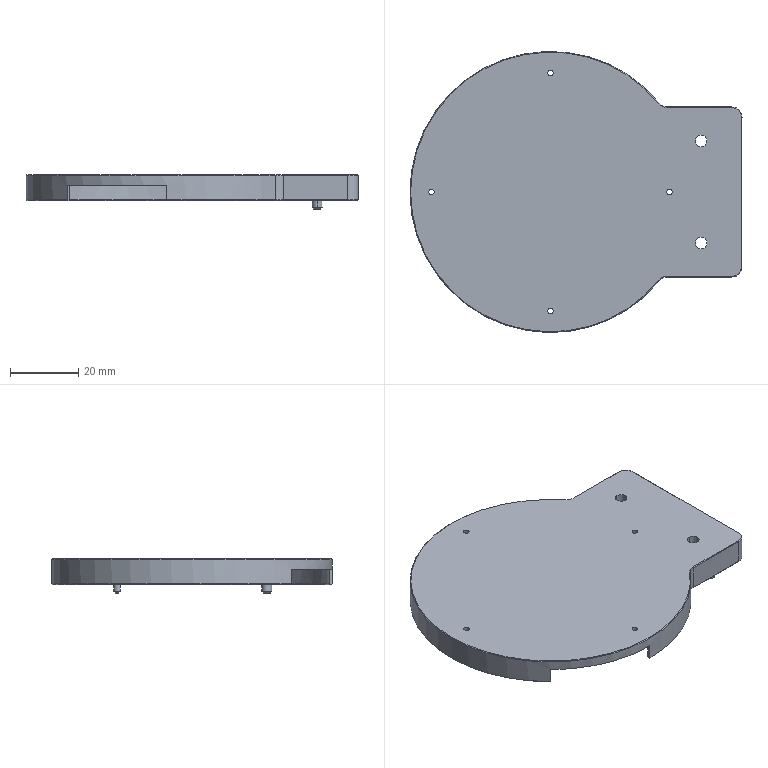Part | 1 solid | 127 faces | box 97.6 x 82.6 x 10 mm | volume 10172 mm3 | cylinder 55 | plane 48 | cone 24 | commonest cylinder face diameters 6 x22 1.6 x8 5 x6 3.4 x4 4 x4 82.6 x4